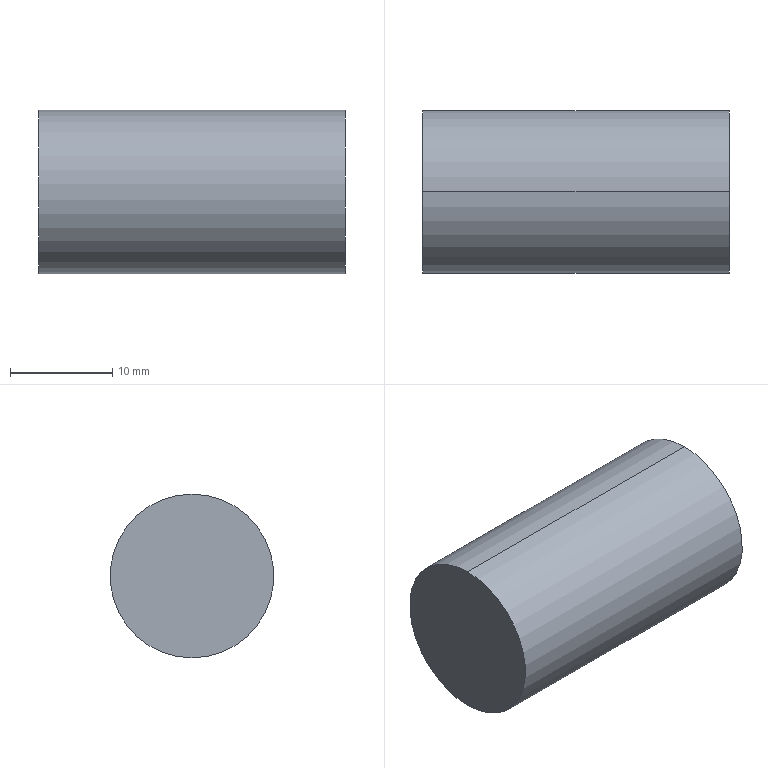Part | SolidWorks | features BaseBody 1 | 1 solid | 4 faces | box 30 x 15.999 x 15.999 mm | volume 6031 mm3 | cylinder 2 | plane 2 | commonest cylinder face diameters 15.999 x2
STEP:
#1=CARTESIAN_POINT('',(-104.,-21.,-160.));
#2=VERTEX_POINT('',#1);
#3=CARTESIAN_POINT('',(-104.,-21.,-176.));
#4=VERTEX_POINT('',#3);
#5=CARTESIAN_POINT('',(-104.,-21.,-168.));
#6=DIRECTION('',(-1.,0.,0.));
#7=DIRECTION('',(0.,0.,1.));
#8=AXIS2_PLACEMENT_3D('',#5,#6,#7);
#9=CIRCLE('',#8,8.);
#10=EDGE_CURVE('',#2,#4,#9,.T.);
#11=ORIENTED_EDGE('',*,*,#10,.T.);
#12=CARTESIAN_POINT('',(-134.,-21.,-176.));
#13=VERTEX_POINT('',#12);
#14=CARTESIAN_POINT('',(-104.,-21.,-176.));
#15=DIRECTION('',(-1.,0.,0.));
#16=VECTOR('',#15,1000.);
#17=LINE('',#14,#16);
#18=EDGE_CURVE('',#4,#13,#17,.T.);
#19=ORIENTED_EDGE('',*,*,#18,.T.);
#20=CARTESIAN_POINT('',(-134.,-21.,-160.));
#21=VERTEX_POINT('',#20);
#22=CARTESIAN_POINT('',(-134.,-21.,-168.));
#23=DIRECTION('',(1.,0.,0.));
#24=DIRECTION('',(0.,0.,1.));
#25=AXIS2_PLACEMENT_3D('',#22,#23,#24);
#26=CIRCLE('',#25,8.);
#27=EDGE_CURVE('',#13,#21,#26,.T.);
#28=ORIENTED_EDGE('',*,*,#27,.T.);
#29=CARTESIAN_POINT('',(-104.,-21.,-160.));
#30=DIRECTION('',(-1.,0.,0.));
#31=VECTOR('',#30,1000.);
#32=LINE('',#29,#31);
#33=EDGE_CURVE('',#2,#21,#32,.T.);
#34=ORIENTED_EDGE('',*,*,#33,.F.);
#35=EDGE_LOOP('',(#11,#19,#28,#34));
#36=FACE_OUTER_BOUND('',#35,.T.);
#37=CARTESIAN_POINT('',(-104.,-21.,-168.));
#38=DIRECTION('',(-1.,0.,0.));
#39=DIRECTION('',(0.,0.,1.));
#40=AXIS2_PLACEMENT_3D('',#37,#38,#39);
#41=CYLINDRICAL_SURFACE('',#40,8.);
#42=ADVANCED_FACE('',(#36),#41,.T.);
#43=ORIENTED_EDGE('',*,*,#18,.F.);
#44=CARTESIAN_POINT('',(-104.,-21.,-168.));
#45=DIRECTION('',(-1.,0.,0.));
#46=DIRECTION('',(0.,0.,1.));
#47=AXIS2_PLACEMENT_3D('',#44,#45,#46);
#48=CIRCLE('',#47,8.);
#49=EDGE_CURVE('',#4,#2,#48,.T.);
#50=ORIENTED_EDGE('',*,*,#49,.T.);
#51=ORIENTED_EDGE('',*,*,#33,.T.);
#52=CARTESIAN_POINT('',(-134.,-21.,-168.));
#53=DIRECTION('',(1.,0.,0.));
#54=DIRECTION('',(0.,0.,1.));
#55=AXIS2_PLACEMENT_3D('',#52,#53,#54);
#56=CIRCLE('',#55,8.);
#57=EDGE_CURVE('',#21,#13,#56,.T.);
#58=ORIENTED_EDGE('',*,*,#57,.T.);
#59=EDGE_LOOP('',(#43,#50,#51,#58));
#60=FACE_OUTER_BOUND('',#59,.T.);
#61=CARTESIAN_POINT('',(-104.,-21.,-168.));
#62=DIRECTION('',(-1.,0.,0.));
#63=DIRECTION('',(0.,0.,1.));
#64=AXIS2_PLACEMENT_3D('',#61,#62,#63);
#65=CYLINDRICAL_SURFACE('',#64,8.);
#66=ADVANCED_FACE('',(#60),#65,.T.);
#67=ORIENTED_EDGE('',*,*,#10,.F.);
#68=ORIENTED_EDGE('',*,*,#49,.F.);
#69=EDGE_LOOP('',(#67,#68));
#70=FACE_OUTER_BOUND('',#69,.T.);
#71=CARTESIAN_POINT('',(-104.,-21.,-168.));
#72=DIRECTION('',(1.,0.,0.));
#73=DIRECTION('',(0.,0.,-1.));
#74=AXIS2_PLACEMENT_3D('',#71,#72,#73);
#75=PLANE('',#74);
#76=ADVANCED_FACE('',(#70),#75,.T.);
#77=ORIENTED_EDGE('',*,*,#57,.F.);
#78=ORIENTED_EDGE('',*,*,#27,.F.);
#79=EDGE_LOOP('',(#77,#78));
#80=FACE_OUTER_BOUND('',#79,.T.);
#81=CARTESIAN_POINT('',(-134.,-21.,-168.));
#82=DIRECTION('',(1.,0.,0.));
#83=DIRECTION('',(0.,0.,-1.));
#84=AXIS2_PLACEMENT_3D('',#81,#82,#83);
#85=PLANE('',#84);
#86=ADVANCED_FACE('',(#80),#85,.F.);
#87=CLOSED_SHELL('',(#42,#66,#76,#86));
#88=MANIFOLD_SOLID_BREP('',#87);
#89=CARTESIAN_POINT('',(0.,0.,0.));
#90=DIRECTION('',(0.,0.,1.));
#91=DIRECTION('',(1.,0.,0.));
#92=AXIS2_PLACEMENT_3D('',#89,#90,#91);
#93=(LENGTH_UNIT()NAMED_UNIT(*)SI_UNIT(.MILLI.,.METRE.));
#94=UNCERTAINTY_MEASURE_WITH_UNIT(LENGTH_MEASURE(0.00001),#93,'','');
#95=(NAMED_UNIT(*)PLANE_ANGLE_UNIT()SI_UNIT($,.RADIAN.));
#96=(NAMED_UNIT(*)SI_UNIT($,.STERADIAN.)SOLID_ANGLE_UNIT());
#97=(GEOMETRIC_REPRESENTATION_CONTEXT(3)GLOBAL_UNCERTAINTY_ASSIGNED_CONTEXT((#94))GLOBAL_UNIT_ASSIGNED_CONTEXT((#93,#95,#96))REPRESENTATION_CONTEXT('',''));
#98=ADVANCED_BREP_SHAPE_REPRESENTATION('',(#88,#92),#97);